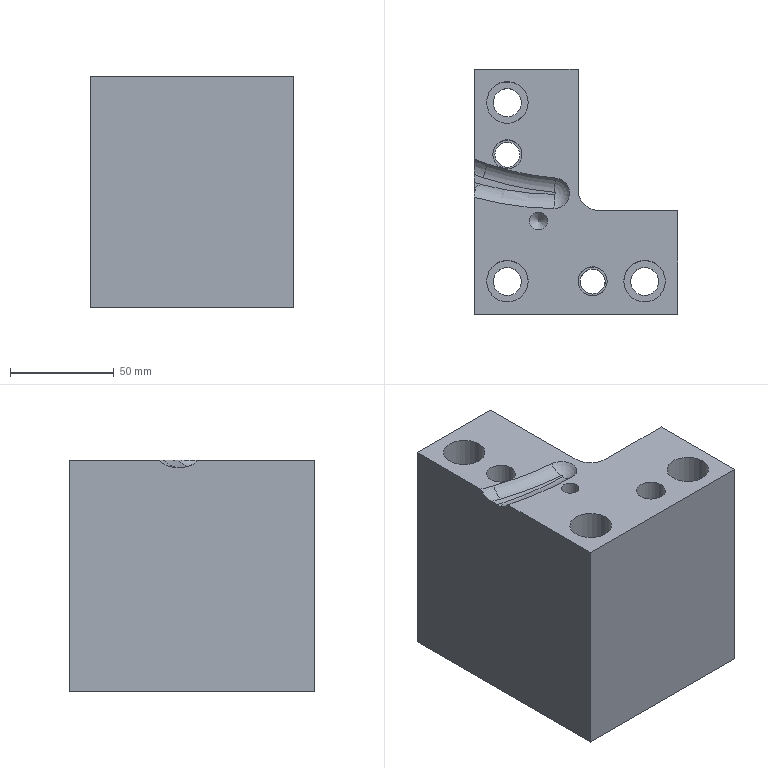Part | NX | features solid 2 | 1 solid | 38 faces | box 98 x 118 x 111.566 mm | volume 796190 mm3 | cylinder 16 | plane 14 | cone 3 | torus 3 | spline 2 | commonest cylinder face diameters 8.5 x5 20 x4 13.5 x3 12.001 x2 14 x2
STEP:
#1=CARTESIAN_POINT('',(1477.25,-202.,-16.5));
#2=VERTEX_POINT('',#1);
#3=CARTESIAN_POINT('',(1473.,-202.,-16.5));
#4=DIRECTION('',(0.,0.,1.));
#5=DIRECTION('',(1.,0.,0.));
#6=AXIS2_PLACEMENT_3D('',#3,#4,#5);
#7=CIRCLE('',#6,4.25);
#8=EDGE_CURVE('',#2,#2,#7,.T.);
#9=ORIENTED_EDGE('',*,*,#8,.F.);
#10=EDGE_LOOP('',(#9));
#11=FACE_BOUND('',#10,.T.);
#12=CARTESIAN_POINT('',(1442.,-190.687,-16.5));
#13=VERTEX_POINT('',#12);
#14=CARTESIAN_POINT('',(1480.409,-196.092,-16.5));
#15=VERTEX_POINT('',#14);
#16=CARTESIAN_POINT('',(1482.477,-42.232,-16.5));
#17=DIRECTION('',(0.,-0.000000004,1.));
#18=DIRECTION('',(0.,-1.,-0.000000004));
#19=AXIS2_PLACEMENT_3D('',#16,#17,#18);
#20=CIRCLE('',#19,153.874);
#21=EDGE_CURVE('',#13,#15,#20,.T.);
#22=ORIENTED_EDGE('',*,*,#21,.F.);
#23=CARTESIAN_POINT('',(1442.,-247.,-16.5));
#24=VERTEX_POINT('',#23);
#25=CARTESIAN_POINT('',(1442.,-125.,-16.5));
#26=DIRECTION('',(0.,1.,0.));
#27=VECTOR('',#26,1000.);
#28=LINE('',#25,#27);
#29=EDGE_CURVE('',#24,#13,#28,.T.);
#30=ORIENTED_EDGE('',*,*,#29,.F.);
#31=CARTESIAN_POINT('',(1540.,-247.,-16.5));
#32=VERTEX_POINT('',#31);
#33=CARTESIAN_POINT('',(1555.5,-247.,-16.5));
#34=DIRECTION('',(-1.,0.,0.));
#35=VECTOR('',#34,1000.);
#36=LINE('',#33,#35);
#37=EDGE_CURVE('',#32,#24,#36,.T.);
#38=ORIENTED_EDGE('',*,*,#37,.F.);
#39=CARTESIAN_POINT('',(1540.,-197.,-16.5));
#40=VERTEX_POINT('',#39);
#41=CARTESIAN_POINT('',(1540.,-125.,-16.5));
#42=DIRECTION('',(0.,1.,0.));
#43=VECTOR('',#42,1000.);
#44=LINE('',#41,#43);
#45=EDGE_CURVE('',#32,#40,#44,.T.);
#46=ORIENTED_EDGE('',*,*,#45,.T.);
#47=CARTESIAN_POINT('',(1502.,-197.,-16.5));
#48=VERTEX_POINT('',#47);
#49=CARTESIAN_POINT('',(1555.5,-197.,-16.5));
#50=DIRECTION('',(-1.,0.,0.));
#51=VECTOR('',#50,1000.);
#52=LINE('',#49,#51);
#53=EDGE_CURVE('',#40,#48,#52,.T.);
#54=ORIENTED_EDGE('',*,*,#53,.T.);
#55=CARTESIAN_POINT('',(1492.,-187.,-16.5));
#56=VERTEX_POINT('',#55);
#57=CARTESIAN_POINT('',(1502.,-187.,-16.5));
#58=DIRECTION('',(0.,0.,-1.));
#59=DIRECTION('',(1.,0.,0.));
#60=AXIS2_PLACEMENT_3D('',#57,#58,#59);
#61=CIRCLE('',#60,10.);
#62=EDGE_CURVE('',#48,#56,#61,.T.);
#63=ORIENTED_EDGE('',*,*,#62,.T.);
#64=CARTESIAN_POINT('',(1492.,-129.,-16.5));
#65=VERTEX_POINT('',#64);
#66=CARTESIAN_POINT('',(1492.,-125.,-16.5));
#67=DIRECTION('',(0.,1.,0.));
#68=VECTOR('',#67,1000.);
#69=LINE('',#66,#68);
#70=EDGE_CURVE('',#56,#65,#69,.T.);
#71=ORIENTED_EDGE('',*,*,#70,.T.);
#72=CARTESIAN_POINT('',(1442.,-129.,-16.5));
#73=VERTEX_POINT('',#72);
#74=CARTESIAN_POINT('',(1555.5,-129.,-16.5));
#75=DIRECTION('',(-1.,0.,0.));
#76=VECTOR('',#75,1000.);
#77=LINE('',#74,#76);
#78=EDGE_CURVE('',#65,#73,#77,.T.);
#79=ORIENTED_EDGE('',*,*,#78,.T.);
#80=CARTESIAN_POINT('',(1442.,-172.34,-16.5));
#81=VERTEX_POINT('',#80);
#82=CARTESIAN_POINT('',(1442.,-125.,-16.5));
#83=DIRECTION('',(0.,1.,0.));
#84=VECTOR('',#83,1000.);
#85=LINE('',#82,#84);
#86=EDGE_CURVE('',#81,#73,#85,.T.);
#87=ORIENTED_EDGE('',*,*,#86,.F.);
#88=CARTESIAN_POINT('',(1448.39,-174.652,-16.5));
#89=VERTEX_POINT('',#88);
#90=CARTESIAN_POINT('',(1448.39,-174.651,-16.5));
#91=CARTESIAN_POINT('',(1446.243,-173.93,-16.5));
#92=CARTESIAN_POINT('',(1444.11,-173.164,-16.5));
#93=CARTESIAN_POINT('',(1442.,-172.34,-16.5));
#94=B_SPLINE_CURVE_WITH_KNOTS('',3,(#90,#91,#92,#93),.UNSPECIFIED.,.F.,.F.,(4,4),(0.,0.006796),.UNSPECIFIED.);
#95=EDGE_CURVE('',#89,#81,#94,.T.);
#96=ORIENTED_EDGE('',*,*,#95,.F.);
#97=CARTESIAN_POINT('',(1481.125,-181.371,-16.5));
#98=VERTEX_POINT('',#97);
#99=CARTESIAN_POINT('',(1492.934,-40.74,-16.5));
#100=DIRECTION('',(0.,-0.000000004,1.));
#101=DIRECTION('',(0.,-1.,-0.000000004));
#102=AXIS2_PLACEMENT_3D('',#99,#100,#101);
#103=CIRCLE('',#102,141.126);
#104=EDGE_CURVE('',#98,#89,#103,.F.);
#105=ORIENTED_EDGE('',*,*,#104,.F.);
#106=CARTESIAN_POINT('',(1480.508,-188.719,-16.5));
#107=DIRECTION('',(0.,-0.000000004,1.));
#108=DIRECTION('',(0.,-1.,-0.000000004));
#109=AXIS2_PLACEMENT_3D('',#106,#107,#108);
#110=CIRCLE('',#109,7.374);
#111=EDGE_CURVE('',#15,#98,#110,.T.);
#112=ORIENTED_EDGE('',*,*,#111,.F.);
#113=EDGE_LOOP('',(#22,#30,#38,#46,#54,#63,#71,#79,#87,#96,#105,#112));
#114=FACE_BOUND('',#113,.T.);
#115=CARTESIAN_POINT('',(1506.,-231.,-16.5));
#116=VERTEX_POINT('',#115);
#117=CARTESIAN_POINT('',(1499.,-231.,-16.5));
#118=DIRECTION('',(0.,0.,1.));
#119=DIRECTION('',(1.,0.,0.));
#120=AXIS2_PLACEMENT_3D('',#117,#118,#119);
#121=CIRCLE('',#120,7.);
#122=EDGE_CURVE('',#116,#116,#121,.T.);
#123=ORIENTED_EDGE('',*,*,#122,.F.);
#124=EDGE_LOOP('',(#123));
#125=FACE_BOUND('',#124,.T.);
#126=CARTESIAN_POINT('',(1514.,-231.,-16.5));
#127=VERTEX_POINT('',#126);
#128=CARTESIAN_POINT('',(1524.,-231.,-16.5));
#129=DIRECTION('',(0.,0.,1.));
#130=DIRECTION('',(-1.,0.,0.));
#131=AXIS2_PLACEMENT_3D('',#128,#129,#130);
#132=CIRCLE('',#131,10.);
#133=EDGE_CURVE('',#127,#127,#132,.T.);
#134=ORIENTED_EDGE('',*,*,#133,.F.);
#135=EDGE_LOOP('',(#134));
#136=FACE_BOUND('',#135,.T.);
#137=CARTESIAN_POINT('',(1448.,-145.,-16.5));
#138=VERTEX_POINT('',#137);
#139=CARTESIAN_POINT('',(1458.,-145.,-16.5));
#140=DIRECTION('',(0.,0.,-1.));
#141=DIRECTION('',(-1.,0.,0.));
#142=AXIS2_PLACEMENT_3D('',#139,#140,#141);
#143=CIRCLE('',#142,10.);
#144=EDGE_CURVE('',#138,#138,#143,.T.);
#145=ORIENTED_EDGE('',*,*,#144,.T.);
#146=EDGE_LOOP('',(#145));
#147=FACE_BOUND('',#146,.T.);
#148=CARTESIAN_POINT('',(1465.,-170.,-16.5));
#149=VERTEX_POINT('',#148);
#150=CARTESIAN_POINT('',(1458.,-170.,-16.5));
#151=DIRECTION('',(0.,0.,1.));
#152=DIRECTION('',(1.,0.,0.));
#153=AXIS2_PLACEMENT_3D('',#150,#151,#152);
#154=CIRCLE('',#153,7.);
#155=EDGE_CURVE('',#149,#149,#154,.T.);
#156=ORIENTED_EDGE('',*,*,#155,.F.);
#157=EDGE_LOOP('',(#156));
#158=FACE_BOUND('',#157,.T.);
#159=CARTESIAN_POINT('',(1468.,-231.,-16.5));
#160=VERTEX_POINT('',#159);
#161=CARTESIAN_POINT('',(1458.,-231.,-16.5));
#162=DIRECTION('',(0.,0.,-1.));
#163=DIRECTION('',(1.,0.,0.));
#164=AXIS2_PLACEMENT_3D('',#161,#162,#163);
#165=CIRCLE('',#164,10.);
#166=EDGE_CURVE('',#160,#160,#165,.T.);
#167=ORIENTED_EDGE('',*,*,#166,.T.);
#168=EDGE_LOOP('',(#167));
#169=FACE_BOUND('',#168,.T.);
#170=CARTESIAN_POINT('',(1555.5,-125.,-16.5));
#171=DIRECTION('',(0.,0.,1.));
#172=DIRECTION('',(-1.,0.,0.));
#173=AXIS2_PLACEMENT_3D('',#170,#171,#172);
#174=PLANE('',#173);
#175=ADVANCED_FACE('',(#11,#114,#125,#136,#147,#158,#169),#174,.T.);
#176=ORIENTED_EDGE('',*,*,#78,.F.);
#177=CARTESIAN_POINT('',(1492.,-129.,-128.));
#178=VERTEX_POINT('',#177);
#179=CARTESIAN_POINT('',(1492.,-129.,-88.5));
#180=DIRECTION('',(0.,0.,-1.));
#181=VECTOR('',#180,1000.);
#182=LINE('',#179,#181);
#183=EDGE_CURVE('',#65,#178,#182,.T.);
#184=ORIENTED_EDGE('',*,*,#183,.T.);
#185=CARTESIAN_POINT('',(1442.,-129.,-128.));
#186=VERTEX_POINT('',#185);
#187=CARTESIAN_POINT('',(1555.5,-129.,-128.));
#188=DIRECTION('',(1.,0.,0.));
#189=VECTOR('',#188,1000.);
#190=LINE('',#187,#189);
#191=EDGE_CURVE('',#186,#178,#190,.T.);
#192=ORIENTED_EDGE('',*,*,#191,.F.);
#193=CARTESIAN_POINT('',(1442.,-129.,-88.5));
#194=DIRECTION('',(0.,0.,-1.));
#195=VECTOR('',#194,1000.);
#196=LINE('',#193,#195);
#197=EDGE_CURVE('',#73,#186,#196,.T.);
#198=ORIENTED_EDGE('',*,*,#197,.F.);
#199=EDGE_LOOP('',(#176,#184,#192,#198));
#200=FACE_BOUND('',#199,.T.);
#201=CARTESIAN_POINT('',(1498.5,-129.,-54.));
#202=DIRECTION('',(0.,1.,0.));
#203=DIRECTION('',(0.,0.,-1.));
#204=AXIS2_PLACEMENT_3D('',#201,#202,#203);
#205=PLANE('',#204);
#206=ADVANCED_FACE('',(#200),#205,.T.);
#207=CARTESIAN_POINT('',(1442.001,-189.111,-18.102));
#208=VERTEX_POINT('',#207);
#209=CARTESIAN_POINT('',(1442.,-189.111,-18.102));
#210=CARTESIAN_POINT('',(1442.,-189.706,-17.636));
#211=CARTESIAN_POINT('',(1442.,-190.232,-17.103));
#212=CARTESIAN_POINT('',(1442.,-190.687,-16.5));
#213=B_SPLINE_CURVE_WITH_KNOTS('',3,(#209,#210,#211,#212),.UNSPECIFIED.,.F.,.F.,(4,4),(0.,0.002247),.UNSPECIFIED.);
#214=EDGE_CURVE('',#208,#13,#213,.T.);
#215=ORIENTED_EDGE('',*,*,#214,.F.);
#216=CARTESIAN_POINT('',(1442.,-183.53,-20.));
#217=VERTEX_POINT('',#216);
#218=CARTESIAN_POINT('',(1442.,-183.53,-20.));
#219=CARTESIAN_POINT('',(1442.,-185.543,-19.997));
#220=CARTESIAN_POINT('',(1442.,-187.524,-19.342));
#221=CARTESIAN_POINT('',(1442.,-189.111,-18.102));
#222=B_SPLINE_CURVE_WITH_KNOTS('',3,(#218,#219,#220,#221),.UNSPECIFIED.,.F.,.F.,(4,4),(0.,0.006019),.UNSPECIFIED.);
#223=EDGE_CURVE('',#217,#208,#222,.T.);
#224=ORIENTED_EDGE('',*,*,#223,.F.);
#225=CARTESIAN_POINT('',(1442.,-179.741,-20.));
#226=VERTEX_POINT('',#225);
#227=CARTESIAN_POINT('',(1442.,-125.,-20.));
#228=DIRECTION('',(0.,1.,0.000000004));
#229=VECTOR('',#228,1000.);
#230=LINE('',#227,#229);
#231=EDGE_CURVE('',#217,#226,#230,.T.);
#232=ORIENTED_EDGE('',*,*,#231,.T.);
#233=CARTESIAN_POINT('',(1442.,-172.34,-16.5));
#234=CARTESIAN_POINT('',(1442.,-174.066,-18.776));
#235=CARTESIAN_POINT('',(1442.,-176.892,-20.024));
#236=CARTESIAN_POINT('',(1442.,-179.741,-20.));
#237=B_SPLINE_CURVE_WITH_KNOTS('',3,(#233,#234,#235,#236),.UNSPECIFIED.,.F.,.F.,(4,4),(0.,0.008439),.UNSPECIFIED.);
#238=EDGE_CURVE('',#81,#226,#237,.T.);
#239=ORIENTED_EDGE('',*,*,#238,.F.);
#240=ORIENTED_EDGE('',*,*,#86,.T.);
#241=ORIENTED_EDGE('',*,*,#197,.T.);
#242=CARTESIAN_POINT('',(1442.,-247.,-128.));
#243=VERTEX_POINT('',#242);
#244=CARTESIAN_POINT('',(1442.,-125.,-128.));
#245=DIRECTION('',(0.,-1.,0.));
#246=VECTOR('',#245,1000.);
#247=LINE('',#244,#246);
#248=EDGE_CURVE('',#186,#243,#247,.T.);
#249=ORIENTED_EDGE('',*,*,#248,.T.);
#250=CARTESIAN_POINT('',(1442.,-247.,-88.5));
#251=DIRECTION('',(0.,0.,1.));
#252=VECTOR('',#251,1000.);
#253=LINE('',#250,#252);
#254=EDGE_CURVE('',#243,#24,#253,.T.);
#255=ORIENTED_EDGE('',*,*,#254,.T.);
#256=ORIENTED_EDGE('',*,*,#29,.T.);
#257=EDGE_LOOP('',(#215,#224,#232,#239,#240,#241,#249,#255,#256));
#258=FACE_BOUND('',#257,.T.);
#259=CARTESIAN_POINT('',(1442.,-125.,-88.5));
#260=DIRECTION('',(-1.,0.,0.));
#261=DIRECTION('',(0.,0.,-1.));
#262=AXIS2_PLACEMENT_3D('',#259,#260,#261);
#263=PLANE('',#262);
#264=ADVANCED_FACE('',(#258),#263,.T.);
#265=CARTESIAN_POINT('',(1492.,-158.,-27.25));
#266=VERTEX_POINT('',#265);
#267=CARTESIAN_POINT('',(1492.,-158.,-31.5));
#268=DIRECTION('',(-1.,0.,0.));
#269=DIRECTION('',(0.,0.,1.));
#270=AXIS2_PLACEMENT_3D('',#267,#268,#269);
#271=CIRCLE('',#270,4.25);
#272=EDGE_CURVE('',#266,#266,#271,.T.);
#273=ORIENTED_EDGE('',*,*,#272,.T.);
#274=EDGE_LOOP('',(#273));
#275=FACE_BOUND('',#274,.T.);
#276=CARTESIAN_POINT('',(1492.,-158.,-72.25));
#277=VERTEX_POINT('',#276);
#278=CARTESIAN_POINT('',(1492.,-158.,-76.5));
#279=DIRECTION('',(-1.,0.,0.));
#280=DIRECTION('',(0.,0.,1.));
#281=AXIS2_PLACEMENT_3D('',#278,#279,#280);
#282=CIRCLE('',#281,4.25);
#283=EDGE_CURVE('',#277,#277,#282,.T.);
#284=ORIENTED_EDGE('',*,*,#283,.T.);
#285=EDGE_LOOP('',(#284));
#286=FACE_BOUND('',#285,.T.);
#287=ORIENTED_EDGE('',*,*,#183,.F.);
#288=ORIENTED_EDGE('',*,*,#70,.F.);
#289=CARTESIAN_POINT('',(1492.,-187.,-128.));
#290=VERTEX_POINT('',#289);
#291=CARTESIAN_POINT('',(1492.,-187.,-113.));
#292=DIRECTION('',(0.,0.,-1.));
#293=VECTOR('',#292,1000.);
#294=LINE('',#291,#293);
#295=EDGE_CURVE('',#56,#290,#294,.T.);
#296=ORIENTED_EDGE('',*,*,#295,.T.);
#297=CARTESIAN_POINT('',(1492.,-125.,-128.));
#298=DIRECTION('',(0.,-1.,0.));
#299=VECTOR('',#298,1000.);
#300=LINE('',#297,#299);
#301=EDGE_CURVE('',#178,#290,#300,.T.);
#302=ORIENTED_EDGE('',*,*,#301,.F.);
#303=EDGE_LOOP('',(#287,#288,#296,#302));
#304=FACE_BOUND('',#303,.T.);
#305=CARTESIAN_POINT('',(1492.,-125.,-88.5));
#306=DIRECTION('',(-1.,0.,0.));
#307=DIRECTION('',(0.,0.,-1.));
#308=AXIS2_PLACEMENT_3D('',#305,#306,#307);
#309=PLANE('',#308);
#310=ADVANCED_FACE('',(#275,#286,#304),#309,.F.);
#311=CARTESIAN_POINT('',(1492.999,-231.,-128.));
#312=VERTEX_POINT('',#311);
#313=CARTESIAN_POINT('',(1499.,-231.,-128.));
#314=DIRECTION('',(0.,0.,-1.));
#315=DIRECTION('',(-1.,0.,0.));
#316=AXIS2_PLACEMENT_3D('',#313,#314,#315);
#317=CIRCLE('',#316,6.);
#318=EDGE_CURVE('',#312,#312,#317,.T.);
#319=ORIENTED_EDGE('',*,*,#318,.F.);
#320=EDGE_LOOP('',(#319));
#321=FACE_BOUND('',#320,.T.);
#322=CARTESIAN_POINT('',(1517.25,-231.,-128.));
#323=VERTEX_POINT('',#322);
#324=CARTESIAN_POINT('',(1524.,-231.,-128.));
#325=DIRECTION('',(0.,0.,-1.));
#326=DIRECTION('',(-1.,0.,0.));
#327=AXIS2_PLACEMENT_3D('',#324,#325,#326);
#328=CIRCLE('',#327,6.75);
#329=EDGE_CURVE('',#323,#323,#328,.T.);
#330=ORIENTED_EDGE('',*,*,#329,.F.);
#331=EDGE_LOOP('',(#330));
#332=FACE_BOUND('',#331,.T.);
#333=CARTESIAN_POINT('',(1451.25,-231.,-128.));
#334=VERTEX_POINT('',#333);
#335=CARTESIAN_POINT('',(1458.,-231.,-128.));
#336=DIRECTION('',(0.,0.,-1.));
#337=DIRECTION('',(-1.,0.,0.));
#338=AXIS2_PLACEMENT_3D('',#335,#336,#337);
#339=CIRCLE('',#338,6.75);
#340=EDGE_CURVE('',#334,#334,#339,.T.);
#341=ORIENTED_EDGE('',*,*,#340,.F.);
#342=EDGE_LOOP('',(#341));
#343=FACE_BOUND('',#342,.T.);
#344=CARTESIAN_POINT('',(1451.999,-170.,-128.));
#345=VERTEX_POINT('',#344);
#346=CARTESIAN_POINT('',(1458.,-170.,-128.));
#347=DIRECTION('',(0.,0.,-1.));
#348=DIRECTION('',(-1.,0.,0.));
#349=AXIS2_PLACEMENT_3D('',#346,#347,#348);
#350=CIRCLE('',#349,6.);
#351=EDGE_CURVE('',#345,#345,#350,.T.);
#352=ORIENTED_EDGE('',*,*,#351,.F.);
#353=EDGE_LOOP('',(#352));
#354=FACE_BOUND('',#353,.T.);
#355=CARTESIAN_POINT('',(1451.25,-145.,-128.));
#356=VERTEX_POINT('',#355);
#357=CARTESIAN_POINT('',(1458.,-145.,-128.));
#358=DIRECTION('',(0.,0.,-1.));
#359=DIRECTION('',(-1.,0.,0.));
#360=AXIS2_PLACEMENT_3D('',#357,#358,#359);
#361=CIRCLE('',#360,6.75);
#362=EDGE_CURVE('',#356,#356,#361,.T.);
#363=ORIENTED_EDGE('',*,*,#362,.F.);
#364=EDGE_LOOP('',(#363));
#365=FACE_BOUND('',#364,.T.);
#366=ORIENTED_EDGE('',*,*,#248,.F.);
#367=ORIENTED_EDGE('',*,*,#191,.T.);
#368=ORIENTED_EDGE('',*,*,#301,.T.);
#369=CARTESIAN_POINT('',(1502.,-197.,-128.));
#370=VERTEX_POINT('',#369);
#371=CARTESIAN_POINT('',(1502.,-187.,-128.));
#372=DIRECTION('',(0.,0.,1.));
#373=DIRECTION('',(-1.,0.,0.));
#374=AXIS2_PLACEMENT_3D('',#371,#372,#373);
#375=CIRCLE('',#374,10.);
#376=EDGE_CURVE('',#290,#370,#375,.T.);
#377=ORIENTED_EDGE('',*,*,#376,.T.);
#378=CARTESIAN_POINT('',(1540.,-197.,-128.));
#379=VERTEX_POINT('',#378);
#380=CARTESIAN_POINT('',(1555.5,-197.,-128.));
#381=DIRECTION('',(1.,0.,0.));
#382=VECTOR('',#381,1000.);
#383=LINE('',#380,#382);
#384=EDGE_CURVE('',#370,#379,#383,.T.);
#385=ORIENTED_EDGE('',*,*,#384,.T.);
#386=CARTESIAN_POINT('',(1540.,-247.,-128.));
#387=VERTEX_POINT('',#386);
#388=CARTESIAN_POINT('',(1540.,-125.,-128.));
#389=DIRECTION('',(0.,1.,0.));
#390=VECTOR('',#389,1000.);
#391=LINE('',#388,#390);
#392=EDGE_CURVE('',#387,#379,#391,.T.);
#393=ORIENTED_EDGE('',*,*,#392,.F.);
#394=CARTESIAN_POINT('',(1555.5,-247.,-128.));
#395=DIRECTION('',(1.,0.,0.));
#396=VECTOR('',#395,1000.);
#397=LINE('',#394,#396);
#398=EDGE_CURVE('',#243,#387,#397,.T.);
#399=ORIENTED_EDGE('',*,*,#398,.F.);
#400=EDGE_LOOP('',(#366,#367,#368,#377,#385,#393,#399));
#401=FACE_BOUND('',#400,.T.);
#402=CARTESIAN_POINT('',(1555.5,-125.,-128.));
#403=DIRECTION('',(0.,0.,-1.));
#404=DIRECTION('',(1.,0.,0.));
#405=AXIS2_PLACEMENT_3D('',#402,#403,#404);
#406=PLANE('',#405);
#407=ADVANCED_FACE('',(#321,#332,#343,#354,#365,#401),#406,.T.);
#408=CARTESIAN_POINT('',(1540.,-197.,-88.5));
#409=DIRECTION('',(0.,0.,-1.));
#410=VECTOR('',#409,1000.);
#411=LINE('',#408,#410);
#412=EDGE_CURVE('',#40,#379,#411,.T.);
#413=ORIENTED_EDGE('',*,*,#412,.F.);
#414=ORIENTED_EDGE('',*,*,#45,.F.);
#415=CARTESIAN_POINT('',(1540.,-247.,-54.));
#416=DIRECTION('',(0.,0.,-1.));
#417=VECTOR('',#416,1000.);
#418=LINE('',#415,#417);
#419=EDGE_CURVE('',#32,#387,#418,.T.);
#420=ORIENTED_EDGE('',*,*,#419,.T.);
#421=ORIENTED_EDGE('',*,*,#392,.T.);
#422=EDGE_LOOP('',(#413,#414,#420,#421));
#423=FACE_BOUND('',#422,.T.);
#424=CARTESIAN_POINT('',(1540.,-190.5,-54.));
#425=DIRECTION('',(1.,0.,0.));
#426=DIRECTION('',(0.,0.,1.));
#427=AXIS2_PLACEMENT_3D('',#424,#425,#426);
#428=PLANE('',#427);
#429=ADVANCED_FACE('',(#423),#428,.T.);
#430=ORIENTED_EDGE('',*,*,#398,.T.);
#431=ORIENTED_EDGE('',*,*,#419,.F.);
#432=ORIENTED_EDGE('',*,*,#37,.T.);
#433=ORIENTED_EDGE('',*,*,#254,.F.);
#434=EDGE_LOOP('',(#430,#431,#432,#433));
#435=FACE_BOUND('',#434,.T.);
#436=CARTESIAN_POINT('',(1555.5,-247.,-88.5));
#437=DIRECTION('',(0.,-1.,0.));
#438=DIRECTION('',(0.,0.,1.));
#439=AXIS2_PLACEMENT_3D('',#436,#437,#438);
#440=PLANE('',#439);
#441=ADVANCED_FACE('',(#435),#440,.T.);
#442=CARTESIAN_POINT('',(1525.25,-197.,-76.5));
#443=VERTEX_POINT('',#442);
#444=CARTESIAN_POINT('',(1521.,-197.,-76.5));
#445=DIRECTION('',(0.,-1.,0.));
#446=DIRECTION('',(1.,0.,0.));
#447=AXIS2_PLACEMENT_3D('',#444,#445,#446);
#448=CIRCLE('',#447,4.25);
#449=EDGE_CURVE('',#443,#443,#448,.T.);
#450=ORIENTED_EDGE('',*,*,#449,.T.);
#451=EDGE_LOOP('',(#450));
#452=FACE_BOUND('',#451,.T.);
#453=CARTESIAN_POINT('',(1525.25,-197.,-31.5));
#454=VERTEX_POINT('',#453);
#455=CARTESIAN_POINT('',(1521.,-197.,-31.5));
#456=DIRECTION('',(0.,-1.,0.));
#457=DIRECTION('',(1.,0.,0.));
#458=AXIS2_PLACEMENT_3D('',#455,#456,#457);
#459=CIRCLE('',#458,4.25);
#460=EDGE_CURVE('',#454,#454,#459,.T.);
#461=ORIENTED_EDGE('',*,*,#460,.T.);
#462=EDGE_LOOP('',(#461));
#463=FACE_BOUND('',#462,.T.);
#464=CARTESIAN_POINT('',(1502.,-197.,-16.5));
#465=DIRECTION('',(0.,0.,1.));
#466=VECTOR('',#465,1000.);
#467=LINE('',#464,#466);
#468=EDGE_CURVE('',#370,#48,#467,.T.);
#469=ORIENTED_EDGE('',*,*,#468,.T.);
#470=ORIENTED_EDGE('',*,*,#53,.F.);
#471=ORIENTED_EDGE('',*,*,#412,.T.);
#472=ORIENTED_EDGE('',*,*,#384,.F.);
#473=EDGE_LOOP('',(#469,#470,#471,#472));
#474=FACE_BOUND('',#473,.T.);
#475=CARTESIAN_POINT('',(1555.5,-197.,-88.5));
#476=DIRECTION('',(0.,-1.,0.));
#477=DIRECTION('',(0.,0.,1.));
#478=AXIS2_PLACEMENT_3D('',#475,#476,#477);
#479=PLANE('',#478);
#480=ADVANCED_FACE('',(#452,#463,#474),#479,.F.);
#481=ORIENTED_EDGE('',*,*,#295,.F.);
#482=ORIENTED_EDGE('',*,*,#62,.F.);
#483=ORIENTED_EDGE('',*,*,#468,.F.);
#484=ORIENTED_EDGE('',*,*,#376,.F.);
#485=EDGE_LOOP('',(#481,#482,#483,#484));
#486=FACE_BOUND('',#485,.T.);
#487=CARTESIAN_POINT('',(1502.,-187.,-88.5));
#488=DIRECTION('',(0.,0.,1.));
#489=DIRECTION('',(-1.,0.,0.));
#490=AXIS2_PLACEMENT_3D('',#487,#488,#489);
#491=CYLINDRICAL_SURFACE('',#490,10.);
#492=ADVANCED_FACE('',(#486),#491,.F.);
#493=ORIENTED_EDGE('',*,*,#362,.T.);
#494=EDGE_LOOP('',(#493));
#495=FACE_BOUND('',#494,.T.);
#496=CARTESIAN_POINT('',(1464.75,-145.,-98.));
#497=VERTEX_POINT('',#496);
#498=CARTESIAN_POINT('',(1458.,-145.,-98.));
#499=DIRECTION('',(0.,0.,-1.));
#500=DIRECTION('',(1.,0.,0.));
#501=AXIS2_PLACEMENT_3D('',#498,#499,#500);
#502=CIRCLE('',#501,6.75);
#503=EDGE_CURVE('',#497,#497,#502,.T.);
#504=ORIENTED_EDGE('',*,*,#503,.F.);
#505=EDGE_LOOP('',(#504));
#506=FACE_BOUND('',#505,.T.);
#507=CARTESIAN_POINT('',(1458.,-145.,-29.5));
#508=DIRECTION('',(0.,0.,-1.));
#509=DIRECTION('',(1.,0.,0.));
#510=AXIS2_PLACEMENT_3D('',#507,#508,#509);
#511=CYLINDRICAL_SURFACE('',#510,6.75);
#512=ADVANCED_FACE('',(#495,#506),#511,.F.);
#513=ORIENTED_EDGE('',*,*,#503,.T.);
#514=EDGE_LOOP('',(#513));
#515=FACE_BOUND('',#514,.T.);
#516=CARTESIAN_POINT('',(1448.,-145.,-98.));
#517=VERTEX_POINT('',#516);
#518=CARTESIAN_POINT('',(1458.,-145.,-98.));
#519=DIRECTION('',(0.,0.,-1.));
#520=DIRECTION('',(-1.,0.,0.));
#521=AXIS2_PLACEMENT_3D('',#518,#519,#520);
#522=CIRCLE('',#521,10.);
#523=EDGE_CURVE('',#517,#517,#522,.T.);
#524=ORIENTED_EDGE('',*,*,#523,.F.);
#525=EDGE_LOOP('',(#524));
#526=FACE_BOUND('',#525,.T.);
#527=CARTESIAN_POINT('',(1458.,-145.,-98.));
#528=DIRECTION('',(0.,0.,-1.));
#529=DIRECTION('',(-1.,0.,0.));
#530=AXIS2_PLACEMENT_3D('',#527,#528,#529);
#531=PLANE('',#530);
#532=ADVANCED_FACE('',(#515,#526),#531,.F.);
#533=CARTESIAN_POINT('',(1462.25,-154.052,-29.927));
#534=VERTEX_POINT('',#533);
#535=CARTESIAN_POINT('',(1462.25,-154.052,-33.073));
#536=VERTEX_POINT('',#535);
#537=CARTESIAN_POINT('',(1462.25,-154.052,-29.927));
#538=CARTESIAN_POINT('',(1461.946,-154.194,-30.389));
#539=CARTESIAN_POINT('',(1461.486,-154.373,-31.498));
#540=CARTESIAN_POINT('',(1461.946,-154.195,-32.61));
#541=CARTESIAN_POINT('',(1462.25,-154.052,-33.073));
#542=B_SPLINE_CURVE_WITH_KNOTS('',3,(#537,#538,#539,#540,#541),.UNSPECIFIED.,.F.,.F.,(4,1,4),(0.,0.001696,0.003393),.UNSPECIFIED.);
#543=EDGE_CURVE('',#534,#536,#542,.T.);
#544=ORIENTED_EDGE('',*,*,#543,.T.);
#545=CARTESIAN_POINT('',(1462.25,-154.052,-33.073));
#546=CARTESIAN_POINT('',(1462.613,-153.881,-32.645));
#547=CARTESIAN_POINT('',(1463.069,-153.619,-31.502));
#548=CARTESIAN_POINT('',(1462.614,-153.881,-30.355));
#549=CARTESIAN_POINT('',(1462.25,-154.052,-29.927));
#550=B_SPLINE_CURVE_WITH_KNOTS('',3,(#545,#546,#547,#548,#549),.UNSPECIFIED.,.F.,.F.,(4,1,4),(0.,0.001743,0.003486),.UNSPECIFIED.);
#551=EDGE_CURVE('',#536,#534,#550,.T.);
#552=ORIENTED_EDGE('',*,*,#551,.T.);
#553=EDGE_LOOP('',(#544,#552));
#554=FACE_BOUND('',#553,.T.);
#555=CARTESIAN_POINT('',(1462.25,-154.052,-74.927));
#556=VERTEX_POINT('',#555);
#557=CARTESIAN_POINT('',(1462.25,-154.052,-78.073));
#558=VERTEX_POINT('',#557);
#559=CARTESIAN_POINT('',(1462.25,-154.052,-74.927));
#560=CARTESIAN_POINT('',(1461.946,-154.194,-75.389));
#561=CARTESIAN_POINT('',(1461.486,-154.373,-76.498));
#562=CARTESIAN_POINT('',(1461.946,-154.195,-77.61));
#563=CARTESIAN_POINT('',(1462.25,-154.052,-78.073));
#564=B_SPLINE_CURVE_WITH_KNOTS('',3,(#559,#560,#561,#562,#563),.UNSPECIFIED.,.F.,.F.,(4,1,4),(0.,0.001696,0.003393),.UNSPECIFIED.);
#565=EDGE_CURVE('',#556,#558,#564,.T.);
#566=ORIENTED_EDGE('',*,*,#565,.T.);
#567=CARTESIAN_POINT('',(1462.25,-154.052,-78.073));
#568=CARTESIAN_POINT('',(1462.613,-153.881,-77.645));
#569=CARTESIAN_POINT('',(1463.069,-153.619,-76.502));
#570=CARTESIAN_POINT('',(1462.614,-153.881,-75.355));
#571=CARTESIAN_POINT('',(1462.25,-154.052,-74.927));
#572=B_SPLINE_CURVE_WITH_KNOTS('',3,(#567,#568,#569,#570,#571),.UNSPECIFIED.,.F.,.F.,(4,1,4),(0.,0.001743,0.003486),.UNSPECIFIED.);
#573=EDGE_CURVE('',#558,#556,#572,.T.);
#574=ORIENTED_EDGE('',*,*,#573,.T.);
#575=EDGE_LOOP('',(#566,#574));
#576=FACE_BOUND('',#575,.T.);
#577=ORIENTED_EDGE('',*,*,#523,.T.);
#578=EDGE_LOOP('',(#577));
#579=FACE_BOUND('',#578,.T.);
#580=ORIENTED_EDGE('',*,*,#144,.F.);
#581=EDGE_LOOP('',(#580));
#582=FACE_BOUND('',#581,.T.);
#583=CARTESIAN_POINT('',(1458.,-145.,-16.5));
#584=DIRECTION('',(0.,0.,-1.));
#585=DIRECTION('',(1.,0.,0.));
#586=AXIS2_PLACEMENT_3D('',#583,#584,#585);
#587=CYLINDRICAL_SURFACE('',#586,10.);
#588=ADVANCED_FACE('',(#554,#576,#579,#582),#587,.F.);
#589=ORIENTED_EDGE('',*,*,#351,.T.);
#590=EDGE_LOOP('',(#589));
#591=FACE_BOUND('',#590,.T.);
#592=CARTESIAN_POINT('',(1451.999,-170.,-102.));
#593=VERTEX_POINT('',#592);
#594=CARTESIAN_POINT('',(1458.,-170.,-102.));
#595=DIRECTION('',(0.,0.,-1.));
#596=DIRECTION('',(-1.,0.,0.));
#597=AXIS2_PLACEMENT_3D('',#594,#595,#596);
#598=CIRCLE('',#597,6.);
#599=EDGE_CURVE('',#593,#593,#598,.T.);
#600=ORIENTED_EDGE('',*,*,#599,.F.);
#601=EDGE_LOOP('',(#600));
#602=FACE_BOUND('',#601,.T.);
#603=CARTESIAN_POINT('',(1458.,-170.,-29.5));
#604=DIRECTION('',(0.,0.,-1.));
#605=DIRECTION('',(-1.,0.,0.));
#606=AXIS2_PLACEMENT_3D('',#603,#604,#605);
#607=CYLINDRICAL_SURFACE('',#606,6.);
#608=ADVANCED_FACE('',(#591,#602),#607,.F.);
#609=ORIENTED_EDGE('',*,*,#599,.T.);
#610=EDGE_LOOP('',(#609));
#611=FACE_BOUND('',#610,.T.);
#612=CARTESIAN_POINT('',(1465.,-170.,-102.));
#613=VERTEX_POINT('',#612);
#614=CARTESIAN_POINT('',(1458.,-170.,-102.));
#615=DIRECTION('',(0.,0.,-1.));
#616=DIRECTION('',(1.,0.,0.));
#617=AXIS2_PLACEMENT_3D('',#614,#615,#616);
#618=CIRCLE('',#617,7.);
#619=EDGE_CURVE('',#613,#613,#618,.T.);
#620=ORIENTED_EDGE('',*,*,#619,.F.);
#621=EDGE_LOOP('',(#620));
#622=FACE_BOUND('',#621,.T.);
#623=CARTESIAN_POINT('',(1458.,-170.,-102.));
#624=DIRECTION('',(0.,0.,-1.));
#625=DIRECTION('',(1.,0.,0.));
#626=AXIS2_PLACEMENT_3D('',#623,#624,#625);
#627=PLANE('',#626);
#628=ADVANCED_FACE('',(#611,#622),#627,.F.);
#629=ORIENTED_EDGE('',*,*,#155,.T.);
#630=EDGE_LOOP('',(#629));
#631=FACE_BOUND('',#630,.T.);
#632=ORIENTED_EDGE('',*,*,#619,.T.);
#633=EDGE_LOOP('',(#632));
#634=FACE_BOUND('',#633,.T.);
#635=CARTESIAN_POINT('',(1458.,-170.,-14.5));
#636=DIRECTION('',(0.,0.,-1.));
#637=DIRECTION('',(-1.,0.,0.));
#638=AXIS2_PLACEMENT_3D('',#635,#636,#637);
#639=CYLINDRICAL_SURFACE('',#638,7.);
#640=ADVANCED_FACE('',(#631,#634),#639,.F.);
#641=ORIENTED_EDGE('',*,*,#340,.T.);
#642=EDGE_LOOP('',(#641));
#643=FACE_BOUND('',#642,.T.);
#644=CARTESIAN_POINT('',(1451.25,-231.,-98.));
#645=VERTEX_POINT('',#644);
#646=CARTESIAN_POINT('',(1458.,-231.,-98.));
#647=DIRECTION('',(0.,0.,-1.));
#648=DIRECTION('',(-1.,0.,0.));
#649=AXIS2_PLACEMENT_3D('',#646,#647,#648);
#650=CIRCLE('',#649,6.75);
#651=EDGE_CURVE('',#645,#645,#650,.T.);
#652=ORIENTED_EDGE('',*,*,#651,.F.);
#653=EDGE_LOOP('',(#652));
#654=FACE_BOUND('',#653,.T.);
#655=CARTESIAN_POINT('',(1458.,-231.,-29.5));
#656=DIRECTION('',(0.,0.,-1.));
#657=DIRECTION('',(-1.,0.,0.));
#658=AXIS2_PLACEMENT_3D('',#655,#656,#657);
#659=CYLINDRICAL_SURFACE('',#658,6.75);
#660=ADVANCED_FACE('',(#643,#654),#659,.F.);
#661=ORIENTED_EDGE('',*,*,#651,.T.);
#662=EDGE_LOOP('',(#661));
#663=FACE_BOUND('',#662,.T.);
#664=CARTESIAN_POINT('',(1468.,-231.,-98.));
#665=VERTEX_POINT('',#664);
#666=CARTESIAN_POINT('',(1458.,-231.,-98.));
#667=DIRECTION('',(0.,0.,-1.));
#668=DIRECTION('',(1.,0.,0.));
#669=AXIS2_PLACEMENT_3D('',#666,#667,#668);
#670=CIRCLE('',#669,10.);
#671=EDGE_CURVE('',#665,#665,#670,.T.);
#672=ORIENTED_EDGE('',*,*,#671,.F.);
#673=EDGE_LOOP('',(#672));
#674=FACE_BOUND('',#673,.T.);
#675=CARTESIAN_POINT('',(1458.,-231.,-98.));
#676=DIRECTION('',(0.,0.,-1.));
#677=DIRECTION('',(1.,0.,0.));
#678=AXIS2_PLACEMENT_3D('',#675,#676,#677);
#679=PLANE('',#678);
#680=ADVANCED_FACE('',(#663,#674),#679,.F.);
#681=ORIENTED_EDGE('',*,*,#671,.T.);
#682=EDGE_LOOP('',(#681));
#683=FACE_BOUND('',#682,.T.);
#684=ORIENTED_EDGE('',*,*,#166,.F.);
#685=EDGE_LOOP('',(#684));
#686=FACE_BOUND('',#685,.T.);
#687=CARTESIAN_POINT('',(1458.,-231.,-16.5));
#688=DIRECTION('',(0.,0.,-1.));
#689=DIRECTION('',(-1.,0.,0.));
#690=AXIS2_PLACEMENT_3D('',#687,#688,#689);
#691=CYLINDRICAL_SURFACE('',#690,10.);
#692=ADVANCED_FACE('',(#683,#686),#691,.F.);
#693=ORIENTED_EDGE('',*,*,#329,.T.);
#694=EDGE_LOOP('',(#693));
#695=FACE_BOUND('',#694,.T.);
#696=CARTESIAN_POINT('',(1530.75,-231.,-98.));
#697=VERTEX_POINT('',#696);
#698=CARTESIAN_POINT('',(1524.,-231.,-98.));
#699=DIRECTION('',(0.,0.,1.));
#700=DIRECTION('',(1.,0.,0.));
#701=AXIS2_PLACEMENT_3D('',#698,#699,#700);
#702=CIRCLE('',#701,6.75);
#703=EDGE_CURVE('',#697,#697,#702,.T.);
#704=ORIENTED_EDGE('',*,*,#703,.T.);
#705=EDGE_LOOP('',(#704));
#706=FACE_BOUND('',#705,.T.);
#707=CARTESIAN_POINT('',(1524.,-231.,-29.5));
#708=DIRECTION('',(0.,0.,-1.));
#709=DIRECTION('',(1.,0.,0.));
#710=AXIS2_PLACEMENT_3D('',#707,#708,#709);
#711=CYLINDRICAL_SURFACE('',#710,6.75);
#712=ADVANCED_FACE('',(#695,#706),#711,.F.);
#713=ORIENTED_EDGE('',*,*,#703,.F.);
#714=EDGE_LOOP('',(#713));
#715=FACE_BOUND('',#714,.T.);
#716=CARTESIAN_POINT('',(1514.,-231.,-98.));
#717=VERTEX_POINT('',#716);
#718=CARTESIAN_POINT('',(1524.,-231.,-98.));
#719=DIRECTION('',(0.,0.,1.));
#720=DIRECTION('',(-1.,0.,0.));
#721=AXIS2_PLACEMENT_3D('',#718,#719,#720);
#722=CIRCLE('',#721,10.);
#723=EDGE_CURVE('',#717,#717,#722,.T.);
#724=ORIENTED_EDGE('',*,*,#723,.T.);
#725=EDGE_LOOP('',(#724));
#726=FACE_BOUND('',#725,.T.);
#727=CARTESIAN_POINT('',(1524.,-231.,-98.));
#728=DIRECTION('',(0.,0.,-1.));
#729=DIRECTION('',(-1.,0.,0.));
#730=AXIS2_PLACEMENT_3D('',#727,#728,#729);
#731=PLANE('',#730);
#732=ADVANCED_FACE('',(#715,#726),#731,.F.);
#733=CARTESIAN_POINT('',(1525.25,-221.078,-76.5));
#734=VERTEX_POINT('',#733);
#735=CARTESIAN_POINT('',(1524.489,-220.941,-73.597));
#736=CARTESIAN_POINT('',(1525.757,-221.169,-76.503));
#737=CARTESIAN_POINT('',(1524.492,-220.943,-79.393));
#738=CARTESIAN_POINT('',(1522.457,-221.071,-80.619));
#739=CARTESIAN_POINT('',(1520.735,-221.492,-80.851));
#740=CARTESIAN_POINT('',(1519.156,-222.2,-80.436));
#741=CARTESIAN_POINT('',(1517.894,-223.04,-79.531));
#742=CARTESIAN_POINT('',(1517.003,-223.837,-78.234));
#743=CARTESIAN_POINT('',(1516.624,-224.25,-76.502));
#744=CARTESIAN_POINT('',(1517.002,-223.838,-74.768));
#745=CARTESIAN_POINT('',(1517.894,-223.04,-73.469));
#746=CARTESIAN_POINT('',(1519.155,-222.202,-72.566));
#747=CARTESIAN_POINT('',(1520.723,-221.497,-72.151));
#748=CARTESIAN_POINT('',(1522.438,-221.073,-72.375));
#749=CARTESIAN_POINT('',(1524.489,-220.941,-73.597));
#750=CARTESIAN_POINT('',(1525.757,-221.169,-76.503));
#751=CARTESIAN_POINT('',(1524.492,-220.943,-79.393));
#752=B_SPLINE_CURVE_WITH_KNOTS('',3,(#735,#736,#737,#738,#739,#740,#741,#742,#743,#744,#745,#746,#747,#748,#749,#750,#751),.UNSPECIFIED.,.T.,.F.,(1,1,1,1,1,1,1,1,1,1,1,1,1,1,1,1,1,1,1,1,1),(-0.006943,-0.005207,-0.003471,0.,0.003471,0.005207,0.006943,0.008678,0.01041,0.01215,0.01389,0.01562,0.01736,0.01909,0.02083,0.02256,0.0243,0.02777,0.03124,0.03298,0.03471),.UNSPECIFIED.);
#753=EDGE_CURVE('',#734,#734,#752,.T.);
#754=ORIENTED_EDGE('',*,*,#753,.T.);
#755=EDGE_LOOP('',(#754));
#756=FACE_BOUND('',#755,.T.);
#757=CARTESIAN_POINT('',(1525.25,-221.078,-31.5));
#758=VERTEX_POINT('',#757);
#759=CARTESIAN_POINT('',(1524.489,-220.941,-28.597));
#760=CARTESIAN_POINT('',(1525.757,-221.169,-31.503));
#761=CARTESIAN_POINT('',(1524.492,-220.943,-34.393));
#762=CARTESIAN_POINT('',(1522.457,-221.071,-35.619));
#763=CARTESIAN_POINT('',(1520.735,-221.492,-35.851));
#764=CARTESIAN_POINT('',(1519.156,-222.2,-35.436));
#765=CARTESIAN_POINT('',(1517.894,-223.04,-34.531));
#766=CARTESIAN_POINT('',(1517.003,-223.837,-33.234));
#767=CARTESIAN_POINT('',(1516.624,-224.25,-31.502));
#768=CARTESIAN_POINT('',(1517.002,-223.838,-29.768));
#769=CARTESIAN_POINT('',(1517.894,-223.04,-28.469));
#770=CARTESIAN_POINT('',(1519.155,-222.202,-27.566));
#771=CARTESIAN_POINT('',(1520.723,-221.497,-27.151));
#772=CARTESIAN_POINT('',(1522.438,-221.073,-27.375));
#773=CARTESIAN_POINT('',(1524.489,-220.941,-28.597));
#774=CARTESIAN_POINT('',(1525.757,-221.169,-31.503));
#775=CARTESIAN_POINT('',(1524.492,-220.943,-34.393));
#776=B_SPLINE_CURVE_WITH_KNOTS('',3,(#759,#760,#761,#762,#763,#764,#765,#766,#767,#768,#769,#770,#771,#772,#773,#774,#775),.UNSPECIFIED.,.T.,.F.,(1,1,1,1,1,1,1,1,1,1,1,1,1,1,1,1,1,1,1,1,1),(-0.006943,-0.005207,-0.003471,0.,0.003471,0.005207,0.006943,0.008678,0.01041,0.01215,0.01389,0.01562,0.01736,0.01909,0.02083,0.02256,0.0243,0.02777,0.03124,0.03298,0.03471),.UNSPECIFIED.);
#777=EDGE_CURVE('',#758,#758,#776,.T.);
#778=ORIENTED_EDGE('',*,*,#777,.T.);
#779=EDGE_LOOP('',(#778));
#780=FACE_BOUND('',#779,.T.);
#781=ORIENTED_EDGE('',*,*,#723,.F.);
#782=EDGE_LOOP('',(#781));
#783=FACE_BOUND('',#782,.T.);
#784=ORIENTED_EDGE('',*,*,#133,.T.);
#785=EDGE_LOOP('',(#784));
#786=FACE_BOUND('',#785,.T.);
#787=CARTESIAN_POINT('',(1524.,-231.,-16.5));
#788=DIRECTION('',(0.,0.,-1.));
#789=DIRECTION('',(1.,0.,0.));
#790=AXIS2_PLACEMENT_3D('',#787,#788,#789);
#791=CYLINDRICAL_SURFACE('',#790,10.);
#792=ADVANCED_FACE('',(#756,#780,#783,#786),#791,.F.);
#793=ORIENTED_EDGE('',*,*,#318,.T.);
#794=EDGE_LOOP('',(#793));
#795=FACE_BOUND('',#794,.T.);
#796=CARTESIAN_POINT('',(1499.,-225.,-102.));
#797=VERTEX_POINT('',#796);
#798=CARTESIAN_POINT('',(1499.,-231.,-102.));
#799=DIRECTION('',(0.,0.,-1.));
#800=DIRECTION('',(0.,1.,0.));
#801=AXIS2_PLACEMENT_3D('',#798,#799,#800);
#802=CIRCLE('',#801,6.);
#803=EDGE_CURVE('',#797,#797,#802,.T.);
#804=ORIENTED_EDGE('',*,*,#803,.F.);
#805=EDGE_LOOP('',(#804));
#806=FACE_BOUND('',#805,.T.);
#807=CARTESIAN_POINT('',(1499.,-231.,-29.5));
#808=DIRECTION('',(0.,0.,-1.));
#809=DIRECTION('',(0.,1.,0.));
#810=AXIS2_PLACEMENT_3D('',#807,#808,#809);
#811=CYLINDRICAL_SURFACE('',#810,6.);
#812=ADVANCED_FACE('',(#795,#806),#811,.F.);
#813=ORIENTED_EDGE('',*,*,#803,.T.);
#814=EDGE_LOOP('',(#813));
#815=FACE_BOUND('',#814,.T.);
#816=CARTESIAN_POINT('',(1499.,-238.,-102.));
#817=VERTEX_POINT('',#816);
#818=CARTESIAN_POINT('',(1499.,-231.,-102.));
#819=DIRECTION('',(0.,0.,-1.));
#820=DIRECTION('',(0.,-1.,0.));
#821=AXIS2_PLACEMENT_3D('',#818,#819,#820);
#822=CIRCLE('',#821,7.);
#823=EDGE_CURVE('',#817,#817,#822,.T.);
#824=ORIENTED_EDGE('',*,*,#823,.F.);
#825=EDGE_LOOP('',(#824));
#826=FACE_BOUND('',#825,.T.);
#827=CARTESIAN_POINT('',(1499.,-231.,-102.));
#828=DIRECTION('',(0.,0.,-1.));
#829=DIRECTION('',(0.,-1.,0.));
#830=AXIS2_PLACEMENT_3D('',#827,#828,#829);
#831=PLANE('',#830);
#832=ADVANCED_FACE('',(#815,#826),#831,.F.);
#833=ORIENTED_EDGE('',*,*,#122,.T.);
#834=EDGE_LOOP('',(#833));
#835=FACE_BOUND('',#834,.T.);
#836=ORIENTED_EDGE('',*,*,#823,.T.);
#837=EDGE_LOOP('',(#836));
#838=FACE_BOUND('',#837,.T.);
#839=CARTESIAN_POINT('',(1499.,-231.,-14.5));
#840=DIRECTION('',(0.,0.,-1.));
#841=DIRECTION('',(0.,1.,0.));
#842=AXIS2_PLACEMENT_3D('',#839,#840,#841);
#843=CYLINDRICAL_SURFACE('',#842,7.);
#844=ADVANCED_FACE('',(#835,#838),#843,.F.);
#845=ORIENTED_EDGE('',*,*,#8,.T.);
#846=EDGE_LOOP('',(#845));
#847=FACE_BOUND('',#846,.T.);
#848=CARTESIAN_POINT('',(1468.75,-202.,-43.25));
#849=VERTEX_POINT('',#848);
#850=CARTESIAN_POINT('',(1473.,-202.,-43.25));
#851=DIRECTION('',(0.,0.,1.));
#852=DIRECTION('',(-1.,0.,0.));
#853=AXIS2_PLACEMENT_3D('',#850,#851,#852);
#854=CIRCLE('',#853,4.25);
#855=EDGE_CURVE('',#849,#849,#854,.T.);
#856=ORIENTED_EDGE('',*,*,#855,.F.);
#857=EDGE_LOOP('',(#856));
#858=FACE_BOUND('',#857,.T.);
#859=CARTESIAN_POINT('',(1473.,-202.,-13.5));
#860=DIRECTION('',(0.,0.,-1.));
#861=DIRECTION('',(-1.,0.,0.));
#862=AXIS2_PLACEMENT_3D('',#859,#860,#861);
#863=CYLINDRICAL_SURFACE('',#862,4.25);
#864=ADVANCED_FACE('',(#847,#858),#863,.F.);
#865=CARTESIAN_POINT('',(1473.,-202.,-47.5));
#866=VERTEX_POINT('',#865);
#867=VERTEX_LOOP('',#866);
#868=FACE_BOUND('',#867,.T.);
#869=ORIENTED_EDGE('',*,*,#855,.T.);
#870=EDGE_LOOP('',(#869));
#871=FACE_BOUND('',#870,.T.);
#872=CARTESIAN_POINT('',(1473.,-202.,-43.25));
#873=DIRECTION('',(0.,0.,1.));
#874=DIRECTION('',(-1.,0.,0.));
#875=AXIS2_PLACEMENT_3D('',#872,#873,#874);
#876=CONICAL_SURFACE('',#875,4.25,0.7854);
#877=ADVANCED_FACE('',(#868,#871),#876,.F.);
#878=ORIENTED_EDGE('',*,*,#21,.T.);
#879=CARTESIAN_POINT('',(1480.501,-189.219,-20.));
#880=VERTEX_POINT('',#879);
#881=CARTESIAN_POINT('',(1480.501,-189.219,-11.5));
#882=DIRECTION('',(0.9999,-0.01344,0.));
#883=DIRECTION('',(-0.01344,-0.9999,0.));
#884=AXIS2_PLACEMENT_3D('',#881,#882,#883);
#885=CIRCLE('',#884,8.5);
#886=EDGE_CURVE('',#15,#880,#885,.T.);
#887=ORIENTED_EDGE('',*,*,#886,.T.);
#888=CARTESIAN_POINT('',(1445.542,-184.511,-20.));
#889=VERTEX_POINT('',#888);
#890=CARTESIAN_POINT('',(1482.477,-42.232,-20.));
#891=DIRECTION('',(0.,0.000000004,-1.));
#892=DIRECTION('',(0.,-1.,-0.000000004));
#893=AXIS2_PLACEMENT_3D('',#890,#891,#892);
#894=CIRCLE('',#893,147.);
#895=EDGE_CURVE('',#880,#889,#894,.T.);
#896=ORIENTED_EDGE('',*,*,#895,.T.);
#897=CARTESIAN_POINT('',(1442.316,-186.52,-19.535));
#898=VERTEX_POINT('',#897);
#899=CARTESIAN_POINT('',(1445.54,-184.503,-20.));
#900=CARTESIAN_POINT('',(1445.391,-184.539,-20.));
#901=CARTESIAN_POINT('',(1445.045,-184.689,-19.997));
#902=CARTESIAN_POINT('',(1444.682,-184.84,-19.985));
#903=CARTESIAN_POINT('',(1444.274,-185.007,-19.963));
#904=CARTESIAN_POINT('',(1444.367,-184.974,-19.968));
#905=CARTESIAN_POINT('',(1443.991,-185.096,-19.946));
#906=CARTESIAN_POINT('',(1443.838,-185.146,-19.936));
#907=CARTESIAN_POINT('',(1443.707,-185.189,-19.926));
#908=CARTESIAN_POINT('',(1443.667,-185.202,-19.923));
#909=CARTESIAN_POINT('',(1443.346,-185.328,-19.893));
#910=CARTESIAN_POINT('',(1443.099,-185.472,-19.858));
#911=CARTESIAN_POINT('',(1442.684,-185.699,-19.791));
#912=CARTESIAN_POINT('',(1442.331,-185.964,-19.706));
#913=CARTESIAN_POINT('',(1442.268,-186.348,-19.588));
#914=CARTESIAN_POINT('',(1442.316,-186.52,-19.535));
#915=B_SPLINE_CURVE_WITH_KNOTS('',3,(#899,#900,#901,#902,#903,#904,#905,#906,#907,#908,#909,#910,#911,#912,#913,#914),.UNSPECIFIED.,.F.,.F.,(4,1,1,1,1,1,1,1,1,1,1,1,1,4),(0.,0.125,0.25,0.3125,0.375,0.4062,0.4375,0.4688,0.5,0.5625,0.625,0.75,0.875,1.),.UNSPECIFIED.);
#916=EDGE_CURVE('',#889,#898,#915,.T.);
#917=ORIENTED_EDGE('',*,*,#916,.T.);
#918=CARTESIAN_POINT('',(1442.614,-186.885,-19.436));
#919=VERTEX_POINT('',#918);
#920=CARTESIAN_POINT('',(1442.316,-186.52,-19.535));
#921=CARTESIAN_POINT('',(1442.415,-186.642,-19.503));
#922=CARTESIAN_POINT('',(1442.515,-186.764,-19.47));
#923=CARTESIAN_POINT('',(1442.614,-186.885,-19.436));
#924=B_SPLINE_CURVE_WITH_KNOTS('',3,(#920,#921,#922,#923),.UNSPECIFIED.,.F.,.F.,(4,4),(0.,1.),.UNSPECIFIED.);
#925=EDGE_CURVE('',#898,#919,#924,.T.);
#926=ORIENTED_EDGE('',*,*,#925,.T.);
#927=CARTESIAN_POINT('',(1442.615,-186.885,-19.436));
#928=CARTESIAN_POINT('',(1442.394,-187.689,-19.116));
#929=CARTESIAN_POINT('',(1442.186,-188.443,-18.664));
#930=CARTESIAN_POINT('',(1442.001,-189.111,-18.102));
#931=B_SPLINE_CURVE_WITH_KNOTS('',3,(#927,#928,#929,#930),.UNSPECIFIED.,.F.,.F.,(4,4),(0.,1.),.UNSPECIFIED.);
#932=EDGE_CURVE('',#919,#208,#931,.T.);
#933=ORIENTED_EDGE('',*,*,#932,.T.);
#934=ORIENTED_EDGE('',*,*,#214,.T.);
#935=EDGE_LOOP('',(#878,#887,#896,#917,#926,#933,#934));
#936=FACE_BOUND('',#935,.T.);
#937=CARTESIAN_POINT('',(1482.477,-42.232,-11.5));
#938=DIRECTION('',(0.,-0.000000004,1.));
#939=DIRECTION('',(0.01344,0.9999,0.000000004));
#940=AXIS2_PLACEMENT_3D('',#937,#938,#939);
#941=TOROIDAL_SURFACE('',#940,147.,8.5);
#942=ADVANCED_FACE('',(#936),#941,.F.);
#943=CARTESIAN_POINT('',(1442.,-183.53,-20.));
#944=CARTESIAN_POINT('',(1442.258,-183.604,-20.));
#945=CARTESIAN_POINT('',(1442.668,-183.72,-20.));
#946=CARTESIAN_POINT('',(1443.21,-183.871,-20.));
#947=CARTESIAN_POINT('',(1443.513,-183.956,-20.));
#948=CARTESIAN_POINT('',(1443.806,-184.037,-20.));
#949=CARTESIAN_POINT('',(1443.878,-184.057,-20.));
#950=CARTESIAN_POINT('',(1444.098,-184.118,-20.));
#951=CARTESIAN_POINT('',(1444.539,-184.24,-20.));
#952=CARTESIAN_POINT('',(1445.098,-184.394,-20.));
#953=CARTESIAN_POINT('',(1445.541,-184.516,-20.));
#954=B_SPLINE_CURVE_WITH_KNOTS('',3,(#943,#944,#945,#946,#947,#948,#949,#950,#951,#952,#953),.UNSPECIFIED.,.F.,.F.,(4,1,1,1,1,1,1,1,4),(0.,0.25,0.375,0.4375,0.5,0.5625,0.625,0.75,1.),.UNSPECIFIED.);
#955=EDGE_CURVE('',#217,#889,#954,.T.);
#956=ORIENTED_EDGE('',*,*,#955,.T.);
#957=ORIENTED_EDGE('',*,*,#895,.F.);
#958=CARTESIAN_POINT('',(1480.55,-188.221,-20.));
#959=VERTEX_POINT('',#958);
#960=CARTESIAN_POINT('',(1480.508,-188.719,-20.));
#961=DIRECTION('',(0.,0.000000004,-1.));
#962=DIRECTION('',(0.,-1.,-0.000000004));
#963=AXIS2_PLACEMENT_3D('',#960,#961,#962);
#964=CIRCLE('',#963,0.5);
#965=EDGE_CURVE('',#959,#880,#964,.T.);
#966=ORIENTED_EDGE('',*,*,#965,.F.);
#967=CARTESIAN_POINT('',(1446.373,-181.225,-20.));
#968=VERTEX_POINT('',#967);
#969=CARTESIAN_POINT('',(1492.934,-40.74,-20.));
#970=DIRECTION('',(0.,-0.000000004,1.));
#971=DIRECTION('',(0.,-1.,-0.000000004));
#972=AXIS2_PLACEMENT_3D('',#969,#970,#971);
#973=CIRCLE('',#972,148.);
#974=EDGE_CURVE('',#968,#959,#973,.T.);
#975=ORIENTED_EDGE('',*,*,#974,.F.);
#976=CARTESIAN_POINT('',(1446.373,-181.225,-20.));
#977=CARTESIAN_POINT('',(1444.907,-180.755,-20.));
#978=CARTESIAN_POINT('',(1443.45,-180.26,-20.));
#979=CARTESIAN_POINT('',(1442.,-179.741,-20.));
#980=B_SPLINE_CURVE_WITH_KNOTS('',3,(#976,#977,#978,#979),.UNSPECIFIED.,.F.,.F.,(4,4),(0.,1.),.UNSPECIFIED.);
#981=EDGE_CURVE('',#968,#226,#980,.T.);
#982=ORIENTED_EDGE('',*,*,#981,.T.);
#983=ORIENTED_EDGE('',*,*,#231,.F.);
#984=EDGE_LOOP('',(#956,#957,#966,#975,#982,#983));
#985=FACE_BOUND('',#984,.T.);
#986=CARTESIAN_POINT('',(1430.645,-178.931,-20.));
#987=DIRECTION('',(0.,-0.000000004,1.));
#988=DIRECTION('',(0.9308,-0.3655,-0.000000002));
#989=AXIS2_PLACEMENT_3D('',#986,#987,#988);
#990=PLANE('',#989);
#991=ADVANCED_FACE('',(#985),#990,.T.);
#992=ORIENTED_EDGE('',*,*,#932,.F.);
#993=ORIENTED_EDGE('',*,*,#925,.F.);
#994=ORIENTED_EDGE('',*,*,#916,.F.);
#995=ORIENTED_EDGE('',*,*,#955,.F.);
#996=ORIENTED_EDGE('',*,*,#223,.T.);
#997=EDGE_LOOP('',(#992,#993,#994,#995,#996));
#998=FACE_BOUND('',#997,.T.);
#999=CARTESIAN_POINT('',(1445.55,-184.491,-20.));
#1000=CARTESIAN_POINT('',(1445.539,-184.533,-20.));
#1001=CARTESIAN_POINT('',(1445.505,-184.66,-20.));
#1002=CARTESIAN_POINT('',(1445.442,-184.9,-19.992));
#1003=CARTESIAN_POINT('',(1445.41,-185.019,-19.986));
#1004=CARTESIAN_POINT('',(1445.316,-185.377,-19.959));
#1005=CARTESIAN_POINT('',(1445.253,-185.615,-19.93));
#1006=CARTESIAN_POINT('',(1445.066,-186.323,-19.811));
#1007=CARTESIAN_POINT('',(1444.943,-186.791,-19.688));
#1008=CARTESIAN_POINT('',(1444.586,-188.147,-19.199));
#1009=CARTESIAN_POINT('',(1444.363,-188.997,-18.707));
#1010=CARTESIAN_POINT('',(1444.169,-189.739,-18.079));
#1011=CARTESIAN_POINT('',(1444.361,-184.165,-20.));
#1012=CARTESIAN_POINT('',(1444.349,-184.207,-20.));
#1013=CARTESIAN_POINT('',(1444.315,-184.334,-20.));
#1014=CARTESIAN_POINT('',(1444.25,-184.573,-19.992));
#1015=CARTESIAN_POINT('',(1444.218,-184.692,-19.986));
#1016=CARTESIAN_POINT('',(1444.121,-185.049,-19.958));
#1017=CARTESIAN_POINT('',(1444.057,-185.286,-19.929));
#1018=CARTESIAN_POINT('',(1443.866,-185.993,-19.81));
#1019=CARTESIAN_POINT('',(1443.74,-186.46,-19.688));
#1020=CARTESIAN_POINT('',(1443.374,-187.813,-19.198));
#1021=CARTESIAN_POINT('',(1443.145,-188.66,-18.706));
#1022=CARTESIAN_POINT('',(1442.946,-189.4,-18.079));
#1023=CARTESIAN_POINT('',(1443.17,-183.845,-20.));
#1024=CARTESIAN_POINT('',(1443.158,-183.887,-20.));
#1025=CARTESIAN_POINT('',(1443.123,-184.014,-20.));
#1026=CARTESIAN_POINT('',(1443.056,-184.252,-19.992));
#1027=CARTESIAN_POINT('',(1443.023,-184.371,-19.986));
#1028=CARTESIAN_POINT('',(1442.924,-184.728,-19.958));
#1029=CARTESIAN_POINT('',(1442.859,-184.964,-19.929));
#1030=CARTESIAN_POINT('',(1442.663,-185.669,-19.81));
#1031=CARTESIAN_POINT('',(1442.533,-186.135,-19.687));
#1032=CARTESIAN_POINT('',(1442.158,-187.485,-19.197));
#1033=CARTESIAN_POINT('',(1441.924,-188.33,-18.705));
#1034=CARTESIAN_POINT('',(1441.719,-189.067,-18.079));
#1035=CARTESIAN_POINT('',(1441.985,-183.503,-20.));
#1036=CARTESIAN_POINT('',(1441.973,-183.545,-20.));
#1037=CARTESIAN_POINT('',(1441.937,-183.671,-20.));
#1038=CARTESIAN_POINT('',(1441.869,-183.909,-19.992));
#1039=CARTESIAN_POINT('',(1441.835,-184.027,-19.986));
#1040=CARTESIAN_POINT('',(1441.733,-184.383,-19.958));
#1041=CARTESIAN_POINT('',(1441.665,-184.619,-19.929));
#1042=CARTESIAN_POINT('',(1441.463,-185.322,-19.811));
#1043=CARTESIAN_POINT('',(1441.33,-185.787,-19.688));
#1044=CARTESIAN_POINT('',(1440.943,-187.133,-19.199));
#1045=CARTESIAN_POINT('',(1440.701,-187.976,-18.708));
#1046=CARTESIAN_POINT('',(1440.489,-188.711,-18.082));
#1047=B_SPLINE_SURFACE_WITH_KNOTS('',3,3,((#999,#1000,#1001,#1002,#1003,#1004,#1005,#1006,#1007,#1008,#1009,#1010),(#1011,#1012,#1013,#1014,#1015,#1016,#1017,#1018,#1019,#1020,#1021,#1022),(#1023,#1024,#1025,#1026,#1027,#1028,#1029,#1030,#1031,#1032,#1033,#1034),(#1035,#1036,#1037,#1038,#1039,#1040,#1041,#1042,#1043,#1044,#1045,#1046)),.UNSPECIFIED.,.F.,.F.,.F.,(4,4),(4,2,2,2,2,4),(0.,1.),(0.,0.0625,0.125,0.25,0.5,0.9999),.UNSPECIFIED.);
#1048=ADVANCED_FACE('',(#998),#1047,.T.);
#1049=ORIENTED_EDGE('',*,*,#104,.T.);
#1050=CARTESIAN_POINT('',(1448.39,-174.652,-16.5));
#1051=CARTESIAN_POINT('',(1447.943,-176.157,-18.658));
#1052=CARTESIAN_POINT('',(1447.162,-178.675,-20.));
#1053=CARTESIAN_POINT('',(1446.373,-181.225,-20.));
#1054=B_SPLINE_CURVE_WITH_KNOTS('',3,(#1050,#1051,#1052,#1053),.UNSPECIFIED.,.F.,.F.,(4,4),(0.,1.),.UNSPECIFIED.);
#1055=EDGE_CURVE('',#89,#968,#1054,.T.);
#1056=ORIENTED_EDGE('',*,*,#1055,.T.);
#1057=ORIENTED_EDGE('',*,*,#974,.T.);
#1058=CARTESIAN_POINT('',(1480.55,-188.221,-11.5));
#1059=DIRECTION('',(-0.9965,0.08368,0.));
#1060=DIRECTION('',(-0.08368,-0.9965,0.));
#1061=AXIS2_PLACEMENT_3D('',#1058,#1059,#1060);
#1062=CIRCLE('',#1061,8.5);
#1063=EDGE_CURVE('',#98,#959,#1062,.T.);
#1064=ORIENTED_EDGE('',*,*,#1063,.F.);
#1065=EDGE_LOOP('',(#1049,#1056,#1057,#1064));
#1066=FACE_BOUND('',#1065,.T.);
#1067=CARTESIAN_POINT('',(1492.934,-40.74,-11.5));
#1068=DIRECTION('',(0.,-0.000000004,1.));
#1069=DIRECTION('',(0.08368,0.9965,0.000000004));
#1070=AXIS2_PLACEMENT_3D('',#1067,#1068,#1069);
#1071=TOROIDAL_SURFACE('',#1070,148.,8.5);
#1072=ADVANCED_FACE('',(#1066),#1071,.F.);
#1073=ORIENTED_EDGE('',*,*,#95,.T.);
#1074=ORIENTED_EDGE('',*,*,#238,.T.);
#1075=ORIENTED_EDGE('',*,*,#981,.F.);
#1076=ORIENTED_EDGE('',*,*,#1055,.F.);
#1077=EDGE_LOOP('',(#1073,#1074,#1075,#1076));
#1078=FACE_BOUND('',#1077,.T.);
#1079=CARTESIAN_POINT('',(1448.613,-174.643,-16.389));
#1080=CARTESIAN_POINT('',(1448.553,-174.845,-16.69));
#1081=CARTESIAN_POINT('',(1448.493,-175.039,-16.94));
#1082=CARTESIAN_POINT('',(1448.357,-175.474,-17.445));
#1083=CARTESIAN_POINT('',(1448.283,-175.706,-17.684));
#1084=CARTESIAN_POINT('',(1448.047,-176.44,-18.356));
#1085=CARTESIAN_POINT('',(1447.869,-176.98,-18.741));
#1086=CARTESIAN_POINT('',(1447.485,-178.129,-19.366));
#1087=CARTESIAN_POINT('',(1447.279,-178.737,-19.605));
#1088=CARTESIAN_POINT('',(1446.956,-179.679,-19.844));
#1089=CARTESIAN_POINT('',(1446.847,-179.996,-19.904));
#1090=CARTESIAN_POINT('',(1446.681,-180.475,-19.963));
#1091=CARTESIAN_POINT('',(1446.626,-180.635,-19.977));
#1092=CARTESIAN_POINT('',(1446.514,-180.957,-19.996));
#1093=CARTESIAN_POINT('',(1446.442,-181.163,-20.));
#1094=CARTESIAN_POINT('',(1446.412,-181.247,-20.));
#1095=CARTESIAN_POINT('',(1447.468,-174.278,-16.414));
#1096=CARTESIAN_POINT('',(1447.406,-174.481,-16.716));
#1097=CARTESIAN_POINT('',(1447.345,-174.675,-16.966));
#1098=CARTESIAN_POINT('',(1447.206,-175.111,-17.472));
#1099=CARTESIAN_POINT('',(1447.13,-175.345,-17.713));
#1100=CARTESIAN_POINT('',(1446.889,-176.082,-18.384));
#1101=CARTESIAN_POINT('',(1446.708,-176.624,-18.769));
#1102=CARTESIAN_POINT('',(1446.316,-177.778,-19.39));
#1103=CARTESIAN_POINT('',(1446.106,-178.389,-19.625));
#1104=CARTESIAN_POINT('',(1445.777,-179.334,-19.858));
#1105=CARTESIAN_POINT('',(1445.666,-179.652,-19.915));
#1106=CARTESIAN_POINT('',(1445.497,-180.132,-19.97));
#1107=CARTESIAN_POINT('',(1445.441,-180.293,-19.983));
#1108=CARTESIAN_POINT('',(1445.327,-180.615,-19.999));
#1109=CARTESIAN_POINT('',(1445.255,-180.821,-20.001));
#1110=CARTESIAN_POINT('',(1445.224,-180.905,-20.));
#1111=CARTESIAN_POINT('',(1446.373,-173.914,-16.432));
#1112=CARTESIAN_POINT('',(1446.306,-174.116,-16.736));
#1113=CARTESIAN_POINT('',(1446.242,-174.31,-16.986));
#1114=CARTESIAN_POINT('',(1446.094,-174.746,-17.494));
#1115=CARTESIAN_POINT('',(1446.015,-174.979,-17.734));
#1116=CARTESIAN_POINT('',(1445.762,-175.716,-18.407));
#1117=CARTESIAN_POINT('',(1445.573,-176.259,-18.79));
#1118=CARTESIAN_POINT('',(1445.165,-177.415,-19.408));
#1119=CARTESIAN_POINT('',(1444.948,-178.026,-19.641));
#1120=CARTESIAN_POINT('',(1444.609,-178.972,-19.868));
#1121=CARTESIAN_POINT('',(1444.495,-179.291,-19.923));
#1122=CARTESIAN_POINT('',(1444.322,-179.771,-19.975));
#1123=CARTESIAN_POINT('',(1444.264,-179.931,-19.987));
#1124=CARTESIAN_POINT('',(1444.147,-180.253,-20.001));
#1125=CARTESIAN_POINT('',(1444.073,-180.459,-20.001));
#1126=CARTESIAN_POINT('',(1444.042,-180.543,-19.999));
#1127=CARTESIAN_POINT('',(1444.161,-173.132,-16.453));
#1128=CARTESIAN_POINT('',(1444.089,-173.333,-16.759));
#1129=CARTESIAN_POINT('',(1444.019,-173.526,-17.01));
#1130=CARTESIAN_POINT('',(1443.861,-173.961,-17.52));
#1131=CARTESIAN_POINT('',(1443.776,-174.194,-17.761));
#1132=CARTESIAN_POINT('',(1443.505,-174.93,-18.435));
#1133=CARTESIAN_POINT('',(1443.305,-175.473,-18.818));
#1134=CARTESIAN_POINT('',(1442.874,-176.63,-19.432));
#1135=CARTESIAN_POINT('',(1442.645,-177.242,-19.662));
#1136=CARTESIAN_POINT('',(1442.289,-178.188,-19.882));
#1137=CARTESIAN_POINT('',(1442.17,-178.507,-19.935));
#1138=CARTESIAN_POINT('',(1441.989,-178.986,-19.982));
#1139=CARTESIAN_POINT('',(1441.928,-179.147,-19.992));
#1140=CARTESIAN_POINT('',(1441.807,-179.468,-20.002));
#1141=CARTESIAN_POINT('',(1441.729,-179.674,-20.));
#1142=CARTESIAN_POINT('',(1441.697,-179.758,-19.998));
#1143=CARTESIAN_POINT('',(1443.063,-172.723,-16.457));
#1144=CARTESIAN_POINT('',(1442.988,-172.923,-16.763));
#1145=CARTESIAN_POINT('',(1442.916,-173.115,-17.015));
#1146=CARTESIAN_POINT('',(1442.752,-173.549,-17.525));
#1147=CARTESIAN_POINT('',(1442.664,-173.781,-17.767));
#1148=CARTESIAN_POINT('',(1442.386,-174.516,-18.442));
#1149=CARTESIAN_POINT('',(1442.179,-175.058,-18.825));
#1150=CARTESIAN_POINT('',(1441.737,-176.214,-19.439));
#1151=CARTESIAN_POINT('',(1441.502,-176.825,-19.668));
#1152=CARTESIAN_POINT('',(1441.139,-177.771,-19.886));
#1153=CARTESIAN_POINT('',(1441.016,-178.089,-19.937));
#1154=CARTESIAN_POINT('',(1440.831,-178.568,-19.983));
#1155=CARTESIAN_POINT('',(1440.769,-178.728,-19.993));
#1156=CARTESIAN_POINT('',(1440.646,-179.049,-20.003));
#1157=CARTESIAN_POINT('',(1440.566,-179.255,-20.));
#1158=CARTESIAN_POINT('',(1440.534,-179.338,-19.997));
#1159=CARTESIAN_POINT('',(1441.973,-172.296,-16.455));
#1160=CARTESIAN_POINT('',(1441.895,-172.495,-16.762));
#1161=CARTESIAN_POINT('',(1441.821,-172.686,-17.014));
#1162=CARTESIAN_POINT('',(1441.652,-173.118,-17.525));
#1163=CARTESIAN_POINT('',(1441.562,-173.35,-17.768));
#1164=CARTESIAN_POINT('',(1441.275,-174.083,-18.443));
#1165=CARTESIAN_POINT('',(1441.063,-174.623,-18.827));
#1166=CARTESIAN_POINT('',(1440.61,-175.777,-19.441));
#1167=CARTESIAN_POINT('',(1440.369,-176.387,-19.67));
#1168=CARTESIAN_POINT('',(1439.997,-177.33,-19.887));
#1169=CARTESIAN_POINT('',(1439.872,-177.648,-19.939));
#1170=CARTESIAN_POINT('',(1439.683,-178.126,-19.984));
#1171=CARTESIAN_POINT('',(1439.62,-178.286,-19.994));
#1172=CARTESIAN_POINT('',(1439.494,-178.606,-20.003));
#1173=CARTESIAN_POINT('',(1439.413,-178.811,-20.));
#1174=CARTESIAN_POINT('',(1439.38,-178.894,-19.997));
#1175=B_SPLINE_SURFACE_WITH_KNOTS('',3,3,((#1079,#1080,#1081,#1082,#1083,#1084,#1085,#1086,#1087,#1088,#1089,#1090,#1091,#1092,#1093,#1094),(#1095,#1096,#1097,#1098,#1099,#1100,#1101,#1102,#1103,#1104,#1105,#1106,#1107,#1108,#1109,#1110),(#1111,#1112,#1113,#1114,#1115,#1116,#1117,#1118,#1119,#1120,#1121,#1122,#1123,#1124,#1125,#1126),(#1127,#1128,#1129,#1130,#1131,#1132,#1133,#1134,#1135,#1136,#1137,#1138,#1139,#1140,#1141,#1142),(#1143,#1144,#1145,#1146,#1147,#1148,#1149,#1150,#1151,#1152,#1153,#1154,#1155,#1156,#1157,#1158),(#1159,#1160,#1161,#1162,#1163,#1164,#1165,#1166,#1167,#1168,#1169,#1170,#1171,#1172,#1173,#1174)),.UNSPECIFIED.,.F.,.F.,.F.,(4,2,4),(4,2,2,2,2,2,2,4),(0.,0.5,1.),(0.0001709,0.125,0.25,0.5,0.75,0.875,0.9375,1.),.UNSPECIFIED.);
#1176=ADVANCED_FACE('',(#1078),#1175,.T.);
#1177=ORIENTED_EDGE('',*,*,#111,.T.);
#1178=ORIENTED_EDGE('',*,*,#1063,.T.);
#1179=ORIENTED_EDGE('',*,*,#965,.T.);
#1180=ORIENTED_EDGE('',*,*,#886,.F.);
#1181=EDGE_LOOP('',(#1177,#1178,#1179,#1180));
#1182=FACE_BOUND('',#1181,.T.);
#1183=CARTESIAN_POINT('',(1480.508,-188.719,-11.5));
#1184=DIRECTION('',(0.,-0.000000004,1.));
#1185=DIRECTION('',(0.,-1.,-0.000000004));
#1186=AXIS2_PLACEMENT_3D('',#1183,#1184,#1185);
#1187=DEGENERATE_TOROIDAL_SURFACE('',#1186,0.5,8.5,.T.);
#1188=ADVANCED_FACE('',(#1182),#1187,.F.);
#1189=ORIENTED_EDGE('',*,*,#283,.F.);
#1190=EDGE_LOOP('',(#1189));
#1191=FACE_BOUND('',#1190,.T.);
#1192=CARTESIAN_POINT('',(1462.25,-158.,-76.5));
#1193=DIRECTION('',(-1.,0.,0.));
#1194=DIRECTION('',(0.,0.,1.));
#1195=AXIS2_PLACEMENT_3D('',#1192,#1193,#1194);
#1196=CIRCLE('',#1195,4.25);
#1197=EDGE_CURVE('',#558,#556,#1196,.T.);
#1198=ORIENTED_EDGE('',*,*,#1197,.T.);
#1199=ORIENTED_EDGE('',*,*,#573,.F.);
#1200=EDGE_LOOP('',(#1198,#1199));
#1201=FACE_BOUND('',#1200,.T.);
#1202=CARTESIAN_POINT('',(1492.,-158.,-76.5));
#1203=DIRECTION('',(-1.,0.,0.));
#1204=DIRECTION('',(0.,0.,-1.));
#1205=AXIS2_PLACEMENT_3D('',#1202,#1203,#1204);
#1206=CYLINDRICAL_SURFACE('',#1205,4.25);
#1207=ADVANCED_FACE('',(#1191,#1201),#1206,.F.);
#1208=CARTESIAN_POINT('',(1458.,-158.,-76.5));
#1209=VERTEX_POINT('',#1208);
#1210=VERTEX_LOOP('',#1209);
#1211=FACE_BOUND('',#1210,.T.);
#1212=ORIENTED_EDGE('',*,*,#1197,.F.);
#1213=ORIENTED_EDGE('',*,*,#565,.F.);
#1214=EDGE_LOOP('',(#1212,#1213));
#1215=FACE_BOUND('',#1214,.T.);
#1216=CARTESIAN_POINT('',(1462.25,-158.,-76.5));
#1217=DIRECTION('',(1.,0.,0.));
#1218=DIRECTION('',(0.,0.,1.));
#1219=AXIS2_PLACEMENT_3D('',#1216,#1217,#1218);
#1220=CONICAL_SURFACE('',#1219,4.25,0.7854);
#1221=ADVANCED_FACE('',(#1211,#1215),#1220,.F.);
#1222=ORIENTED_EDGE('',*,*,#272,.F.);
#1223=EDGE_LOOP('',(#1222));
#1224=FACE_BOUND('',#1223,.T.);
#1225=CARTESIAN_POINT('',(1462.25,-158.,-31.5));
#1226=DIRECTION('',(-1.,0.,0.));
#1227=DIRECTION('',(0.,0.,1.));
#1228=AXIS2_PLACEMENT_3D('',#1225,#1226,#1227);
#1229=CIRCLE('',#1228,4.25);
#1230=EDGE_CURVE('',#536,#534,#1229,.T.);
#1231=ORIENTED_EDGE('',*,*,#1230,.T.);
#1232=ORIENTED_EDGE('',*,*,#551,.F.);
#1233=EDGE_LOOP('',(#1231,#1232));
#1234=FACE_BOUND('',#1233,.T.);
#1235=CARTESIAN_POINT('',(1492.,-158.,-31.5));
#1236=DIRECTION('',(-1.,0.,0.));
#1237=DIRECTION('',(0.,0.,-1.));
#1238=AXIS2_PLACEMENT_3D('',#1235,#1236,#1237);
#1239=CYLINDRICAL_SURFACE('',#1238,4.25);
#1240=ADVANCED_FACE('',(#1224,#1234),#1239,.F.);
#1241=CARTESIAN_POINT('',(1458.,-158.,-31.5));
#1242=VERTEX_POINT('',#1241);
#1243=VERTEX_LOOP('',#1242);
#1244=FACE_BOUND('',#1243,.T.);
#1245=ORIENTED_EDGE('',*,*,#1230,.F.);
#1246=ORIENTED_EDGE('',*,*,#543,.F.);
#1247=EDGE_LOOP('',(#1245,#1246));
#1248=FACE_BOUND('',#1247,.T.);
#1249=CARTESIAN_POINT('',(1462.25,-158.,-31.5));
#1250=DIRECTION('',(1.,0.,0.));
#1251=DIRECTION('',(0.,0.,1.));
#1252=AXIS2_PLACEMENT_3D('',#1249,#1250,#1251);
#1253=CONICAL_SURFACE('',#1252,4.25,0.7854);
#1254=ADVANCED_FACE('',(#1244,#1248),#1253,.F.);
#1255=ORIENTED_EDGE('',*,*,#460,.F.);
#1256=EDGE_LOOP('',(#1255));
#1257=FACE_BOUND('',#1256,.T.);
#1258=ORIENTED_EDGE('',*,*,#777,.F.);
#1259=EDGE_LOOP('',(#1258));
#1260=FACE_BOUND('',#1259,.T.);
#1261=CARTESIAN_POINT('',(1521.,-197.,-31.5));
#1262=DIRECTION('',(0.,-1.,0.));
#1263=DIRECTION('',(-1.,0.,0.));
#1264=AXIS2_PLACEMENT_3D('',#1261,#1262,#1263);
#1265=CYLINDRICAL_SURFACE('',#1264,4.25);
#1266=ADVANCED_FACE('',(#1257,#1260),#1265,.F.);
#1267=ORIENTED_EDGE('',*,*,#449,.F.);
#1268=EDGE_LOOP('',(#1267));
#1269=FACE_BOUND('',#1268,.T.);
#1270=ORIENTED_EDGE('',*,*,#753,.F.);
#1271=EDGE_LOOP('',(#1270));
#1272=FACE_BOUND('',#1271,.T.);
#1273=CARTESIAN_POINT('',(1521.,-197.,-76.5));
#1274=DIRECTION('',(0.,-1.,0.));
#1275=DIRECTION('',(-1.,0.,0.));
#1276=AXIS2_PLACEMENT_3D('',#1273,#1274,#1275);
#1277=CYLINDRICAL_SURFACE('',#1276,4.25);
#1278=ADVANCED_FACE('',(#1269,#1272),#1277,.F.);
#1279=CLOSED_SHELL('',(#175,#206,#264,#310,#407,#429,#441,#480,#492,#512,#532,#588,#608,#628,#640,#660,#680,#692,#712,#732,#792,#812,#832,#844,#864,#877,#942,#991,#1048,#1072,#1176,#1188,#1207,#1221,#1240,#1254,#1266,#1278));
#1280=MANIFOLD_SOLID_BREP('',#1279);
#1281=(LENGTH_UNIT()NAMED_UNIT(*)SI_UNIT(.MILLI.,.METRE.));
#1282=UNCERTAINTY_MEASURE_WITH_UNIT(LENGTH_MEASURE(0.103),#1281,'','');
#1283=(NAMED_UNIT(*)PLANE_ANGLE_UNIT()SI_UNIT($,.RADIAN.));
#1284=(NAMED_UNIT(*)SI_UNIT($,.STERADIAN.)SOLID_ANGLE_UNIT());
#1285=(GEOMETRIC_REPRESENTATION_CONTEXT(3)GLOBAL_UNCERTAINTY_ASSIGNED_CONTEXT((#1282))GLOBAL_UNIT_ASSIGNED_CONTEXT((#1281,#1283,#1284))REPRESENTATION_CONTEXT('',''));
#1286=ADVANCED_BREP_SHAPE_REPRESENTATION('',(#1280),#1285);